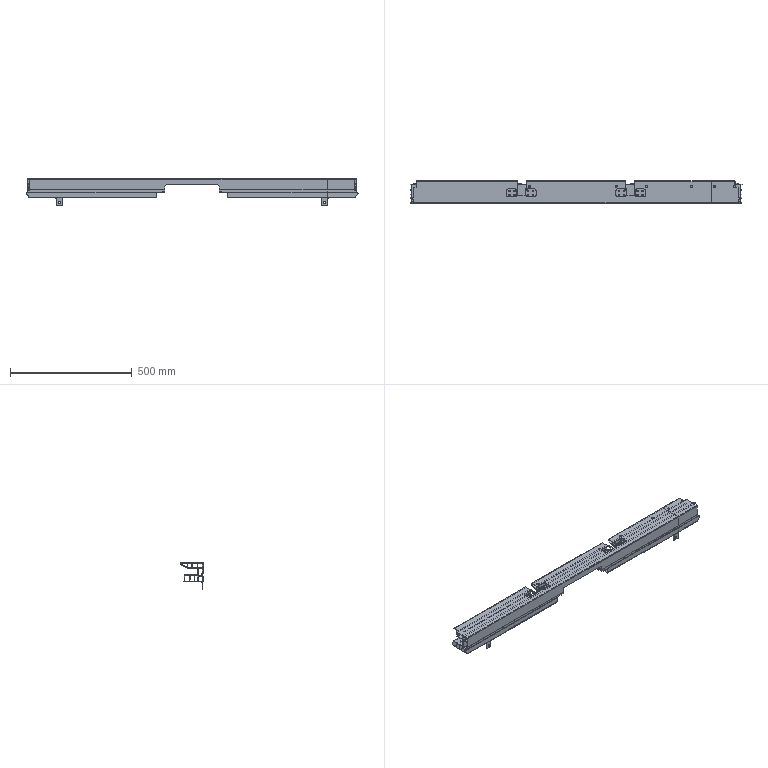NC program | NX | posted with a generic post | part box 1365 x 90.95 x 108.501 mm
Lines 19321 to 19528 of 23380:
(DRILLING_COPY_2 , TOOL : D6A45)
N38604 T07 M6
N38606 G54
N38608 G17 G0 G90 X-658.801 Y42. B0. C0. S3500 M3
N38610 G43 Z30. H7
N38612 G94 G81 G98 Z-27.45 F250. R-23.45
N38614 X-638.75 Y43.25
N38616 X638.75
N38618 X658.801 Y42.
N38620 G80
N38622 G0 X658.801 Y42. Z30.
N38624 M5
(DRILLING_COPY_COPY_1 , TOOL : 7.1ZT)
N38626 T17 M6
N38628 G54
N38630 G17 G0 G90 X658.801 Y42. B0. C0. S1500 M3
N38632 G43 Z30. H17
N38634 G94 G83 G98 Z-32.053 F150. Q4. R-23.45
N38636 X-658.801
N38638 G80
N38640 G0 X-658.801 Y42. Z30.
(DRILLING_COPY_COPY_1_COPY , TOOL : 7.1ZT)
N38642 X-638.75 Y43.25
N38644 G83 Z-50.553 F150. Q4. R-23.45
N38646 X638.75
N38648 G80
N38650 G0 X638.75 Y43.25 Z30.
N38652 M5
(HOLE_MILLING_COPY , TOOL : D10)
N38654 T10 M6
N38656 G54
N38658 G17 G0 G90 X-638.75 Y43.25 B0. C0. S6000 M3
N38660 G43 Z30. H10
N38662 Z-25.65
N38664 G94 G3 X-640.525 Y45.025 R1.775 F2000.
N38666 X-642.3 Y43.25 R1.775
N38668 X-642.3 Y43.25 Z-26.65 I3.55 J0.
N38670 X-642.3 Y43.25 Z-27.65 I3.55 J0.
N38672 X-642.3 Y43.25 Z-28.65 I3.55 J0.
N38674 X-642.3 Y43.25 Z-29.65 I3.55 J0.
N38676 X-637.653 Y39.874 Z-29.95 R3.55
N38678 X-635.374 Y44.347 R3.55
N38680 X-637.653 Y39.874 R-3.55
N38682 X-636.513 Y42.11 R1.775
N38684 X-638.75 Y43.25 R1.775
N38686 G0 Z30.
N38688 X638.75
N38690 Z-25.65
N38692 G3 X636.975 Y45.025 R1.775
N38694 X635.2 Y43.25 R1.775
N38696 X635.2 Y43.25 Z-26.65 I3.55 J0.
N38698 X635.2 Y43.25 Z-27.65 I3.55 J0.
N38700 X635.2 Y43.25 Z-28.65 I3.55 J0.
N38702 X635.2 Y43.25 Z-29.65 I3.55 J0.
N38704 X639.847 Y39.874 Z-29.95 R3.55
N38706 X642.126 Y44.347 R3.55
N38708 X639.847 Y39.874 R-3.55
N38710 X640.987 Y42.11 R1.775
N38712 X638.75 Y43.25 R1.775
N38714 G0 Z30.
(11_COPY_1 , TOOL : D10)
N38716 X137.616 Y-31. S5500
N38718 Z-24.
N38720 G1 Z-27. F500.
N38722 X138.939 Y-30.266
N38724 G3 X139.454 Y-29.408 R1.
N38726 G1 X139.546 Y-23.913 F1000.
N38728 X139.947 Y-0.917
N38730 X139.949 Y-0.903
N38732 X139.974 Y-0.793
N38734 X139.99 Y3.325
N38736 X139.999 Y3.339
N38738 Y5.474
N38740 X139.995 Y5.641
N38742 X140. Y11.408
N38744 G3 X139.501 Y12.275 R1.
N38746 G1 X138.172 Y13.044
N38748 Z-24.
N38750 G0 X137.615 Y-30.999 Z-37.15
N38752 G1 Z-40.15 F500.
N38754 X138.938 Y-30.266
N38756 G3 X139.453 Y-29.408 R1.
N38758 G1 X139.53 Y-24.972 F1000.
N38760 X139.546 Y-23.913
N38762 X139.948 Y-0.903
N38764 X139.973 Y-0.793
N38766 X139.989 Y3.325
N38768 X139.999 Y3.339
N38770 Y5.474
N38772 X139.994 Y5.641
N38774 X140. Y11.408
N38776 G3 X139.5 Y12.275 R1.
N38778 G1 X138.171 Y13.044
N38780 Z-37.15
N38782 G0 X137.615 Y-30.999 Z-50.3
N38784 G1 Z-53.3 F500.
N38786 X138.938 Y-30.266
N38788 G3 X139.453 Y-29.408 R1.
N38790 G1 X139.53 Y-24.972 F1000.
N38792 X139.546 Y-23.913
N38794 X139.948 Y-0.903
N38796 X139.972 Y-0.793
N38798 X139.989 Y3.325
N38800 X139.999 Y3.339
N38802 Y5.461
N38804 X139.994 Y5.474
N38806 X139.999 Y11.408
N38808 G3 X139.5 Y12.275 R1.
N38810 G1 X138.171 Y13.044
N38812 Z-50.3
N38814 G0 X137.615 Y-31. Z-63.45
N38816 G1 Z-66.45 F500.
N38818 X138.938 Y-30.266
N38820 G3 X139.453 Y-29.408 R1.
N38822 G1 X139.546 Y-23.913 F1000.
N38824 X139.967 Y0.186
N38826 G3 X139.988 Y3.325 R148.211
N38828 G1 X139.999 Y3.339
N38830 Y5.461
N38832 X139.993 Y5.474
N38834 X139.999 Y11.408
N38836 G3 X139.5 Y12.275 R1.
N38838 G1 X138.171 Y13.044
N38840 Z-63.45
N38842 G0 Z30.
N38844 X-138.174
N38846 Z-24.
N38848 G1 Z-27. F500.
N38850 X-139.503 Y12.275
N38852 G3 X-140.002 Y11.408 R1.
N38854 G1 X-139.997 Y5.641 F1000.
N38856 X-140.001 Y5.474
N38858 Y3.339
N38860 X-139.992 Y3.325
N38862 X-139.975 Y-0.793
N38864 X-139.951 Y-0.903
N38866 X-139.949 Y-0.917
N38868 X-139.548 Y-23.913
N38870 X-139.547 Y-24.084
N38872 X-139.454 Y-29.408
N38874 G3 X-138.939 Y-30.266 R1.
N38876 G1 X-137.616 Y-30.999
N38878 Z-24.
N38880 G0 X-138.177 Y13.061 Z-37.15
N38882 G1 Z-40.15 F500.
N38884 X-139.508 Y12.278
N38886 G3 X-140.002 Y11.408 R1.
N38888 G1 X-140.001 Y11.298 F1000.
N38890 X-139.995 Y6.084
N38892 X-139.996 Y5.474
N38894 X-140.001 Y5.461
N38896 Y3.339
N38898 X-139.992 Y3.325
N38900 X-139.974 Y-0.793
N38902 X-139.95 Y-0.903
N38904 X-139.548 Y-23.913
N38906 X-139.547 Y-24.084
N38908 X-139.454 Y-29.408
N38910 G3 X-138.939 Y-30.266 R1.
N38912 G1 X-137.615 Y-30.999
N38914 Z-37.15
N38916 G0 X-138.177 Y13.061 Z-50.3
N38918 G1 Z-53.3 F500.
N38920 X-139.508 Y12.278
N38922 G3 X-140.001 Y11.408 R1.
N38924 G1 X-140. Y11.298 F1000.
N38926 X-139.995 Y6.084
N38928 Y5.474
N38930 X-140.001 Y5.461
N38932 Y3.339
N38934 X-139.991 Y3.325
N38936 X-139.973 Y-0.793
N38938 X-139.95 Y-0.903
N38940 X-139.548 Y-23.913
N38942 X-139.546 Y-24.084
N38944 X-139.453 Y-29.408
N38946 G3 X-138.938 Y-30.266 R1.
N38948 G1 X-137.615 Y-30.999
N38950 Z-50.3
N38952 G0 X-138.176 Y13.061 Z-63.45
N38954 G1 Z-66.45 F500.
N38956 X-139.508 Y12.278
N38958 G3 X-140.001 Y11.408 R1.
N38960 G1 X-140. Y11.298 F1000.
N38962 X-139.994 Y6.084
N38964 X-139.995 Y5.474
N38966 X-140.001 Y5.461
N38968 Y3.339
N38970 X-139.991 Y3.325
N38972 G3 X-139.964 Y-0.093 R179.469
N38974 G1 X-139.548 Y-23.913
N38976 X-139.546 Y-24.084
N38978 X-139.453 Y-29.408
N38980 G3 X-138.938 Y-30.266 R1.
N38982 G1 X-137.614 Y-30.999
N38984 Z-63.45
N38986 G0 Z30.
N38988 M5